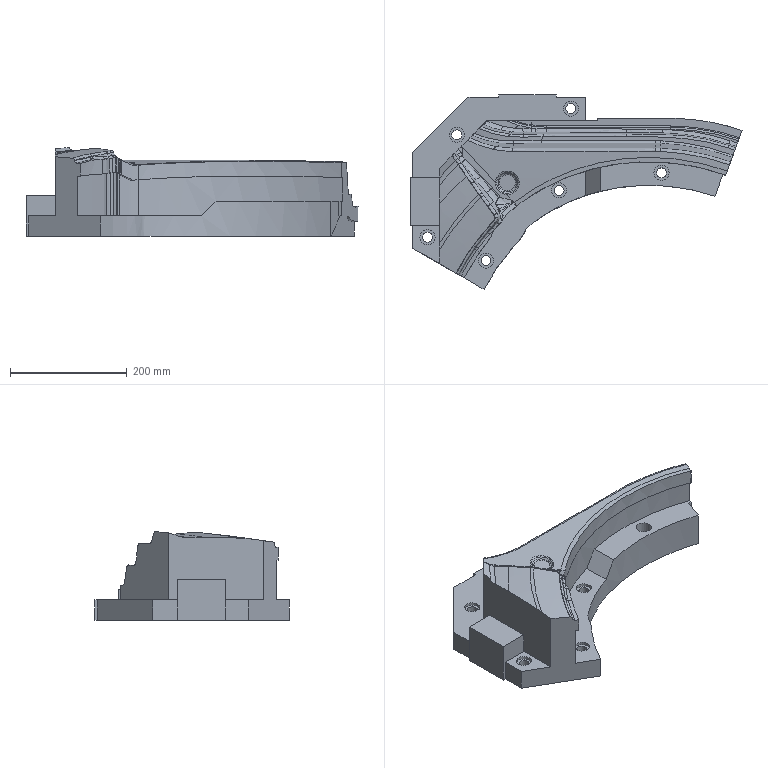Part | NX | features solid 2 | 1 solid | 242 faces | box 567.81 x 333.254 x 151.521 mm | volume 7974180 mm3 | spline 176 | plane 45 | cylinder 21 | commonest cylinder face diameters 17 x7 26 x6 6 x1 6.001 x1 6.003 x1 8 x1